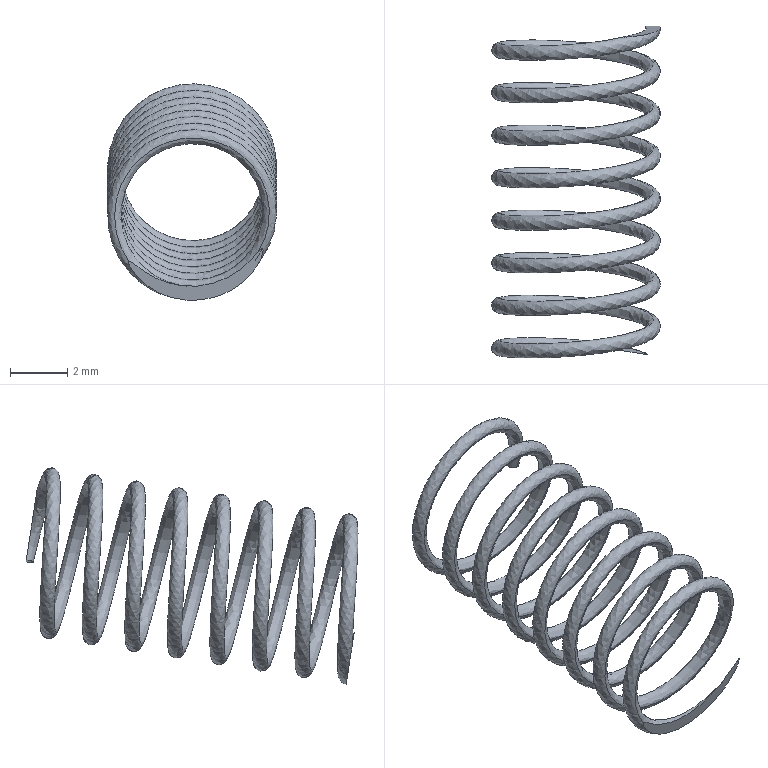Part | SolidWorks | features BaseBody 1 | 1 solid | 5 faces | box 5.9 x 11.576 x 7.553 mm | volume 25.826 mm3 | plane 3 | spline 2